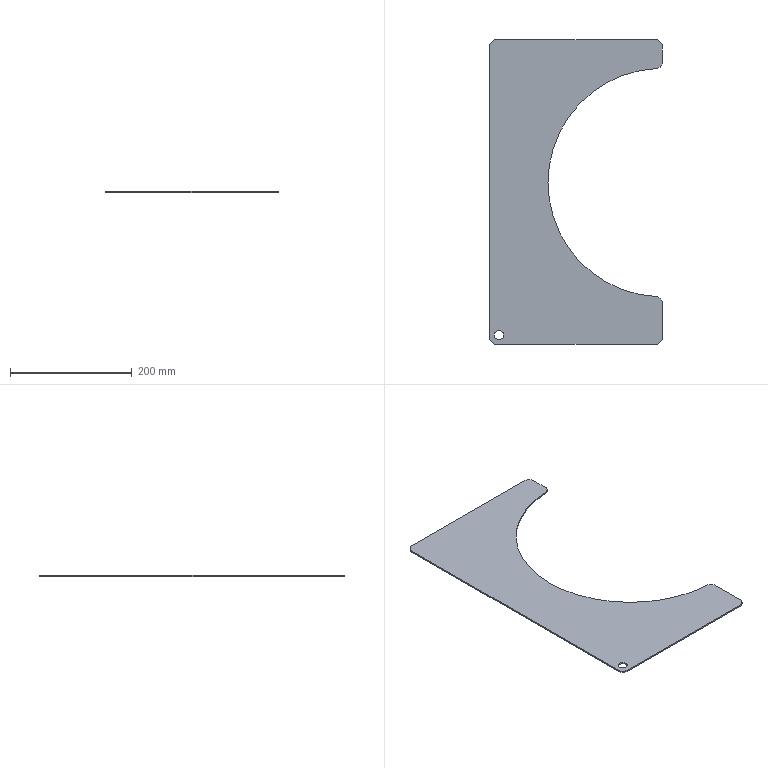Part | SolidWorks | features FlatPattern 1, SMBaseFlange 1, SheetMetal 1 | 1 solid | 17 faces | box 283 x 500 x 2.3 mm | volume 197741 mm3 | cylinder 10 | plane 7 | commonest cylinder face diameters 20 x6 15 x2 375 x2
STEP:
#1=CARTESIAN_POINT('',(7.5,-310.5,2.3));
#2=VERTEX_POINT('',#1);
#3=CARTESIAN_POINT('',(22.5,-310.5,2.3));
#4=VERTEX_POINT('',#3);
#5=CARTESIAN_POINT('',(15.,-310.5,2.3));
#6=DIRECTION('',(0.,0.,1.));
#7=DIRECTION('',(1.,0.,0.));
#8=AXIS2_PLACEMENT_3D('',#5,#6,#7);
#9=CIRCLE('',#8,7.5);
#10=EDGE_CURVE('',#2,#4,#9,.T.);
#11=ORIENTED_EDGE('',*,*,#10,.T.);
#12=CARTESIAN_POINT('',(22.5,-310.5,0.));
#13=VERTEX_POINT('',#12);
#14=CARTESIAN_POINT('',(22.5,-310.5,2.3));
#15=DIRECTION('',(0.,0.,-1.));
#16=VECTOR('',#15,1000.);
#17=LINE('',#14,#16);
#18=EDGE_CURVE('',#4,#13,#17,.T.);
#19=ORIENTED_EDGE('',*,*,#18,.T.);
#20=CARTESIAN_POINT('',(7.5,-310.5,0.));
#21=VERTEX_POINT('',#20);
#22=CARTESIAN_POINT('',(15.,-310.5,0.));
#23=DIRECTION('',(0.,0.,1.));
#24=DIRECTION('',(1.,0.,0.));
#25=AXIS2_PLACEMENT_3D('',#22,#23,#24);
#26=CIRCLE('',#25,7.5);
#27=EDGE_CURVE('',#21,#13,#26,.T.);
#28=ORIENTED_EDGE('',*,*,#27,.F.);
#29=CARTESIAN_POINT('',(7.5,-310.5,2.3));
#30=DIRECTION('',(0.,0.,-1.));
#31=VECTOR('',#30,1000.);
#32=LINE('',#29,#31);
#33=EDGE_CURVE('',#2,#21,#32,.T.);
#34=ORIENTED_EDGE('',*,*,#33,.F.);
#35=EDGE_LOOP('',(#11,#19,#28,#34));
#36=FACE_OUTER_BOUND('',#35,.T.);
#37=CARTESIAN_POINT('',(15.,-310.5,2.3));
#38=DIRECTION('',(0.,0.,-1.));
#39=DIRECTION('',(-1.,0.,0.));
#40=AXIS2_PLACEMENT_3D('',#37,#38,#39);
#41=CYLINDRICAL_SURFACE('',#40,7.5);
#42=ADVANCED_FACE('',(#36),#41,.F.);
#43=CARTESIAN_POINT('',(95.5,-60.,2.3));
#44=VERTEX_POINT('',#43);
#45=CARTESIAN_POINT('',(273.506,127.259,2.3));
#46=VERTEX_POINT('',#45);
#47=CARTESIAN_POINT('',(283.,-60.,2.3));
#48=DIRECTION('',(0.,0.,-1.));
#49=DIRECTION('',(1.,0.,0.));
#50=AXIS2_PLACEMENT_3D('',#47,#48,#49);
#51=CIRCLE('',#50,187.5);
#52=EDGE_CURVE('',#44,#46,#51,.T.);
#53=ORIENTED_EDGE('',*,*,#52,.F.);
#54=CARTESIAN_POINT('',(95.5,-60.,0.));
#55=VERTEX_POINT('',#54);
#56=CARTESIAN_POINT('',(95.5,-60.,2.3));
#57=DIRECTION('',(0.,0.,-1.));
#58=VECTOR('',#57,1000.);
#59=LINE('',#56,#58);
#60=EDGE_CURVE('',#44,#55,#59,.T.);
#61=ORIENTED_EDGE('',*,*,#60,.T.);
#62=CARTESIAN_POINT('',(273.506,127.259,0.));
#63=VERTEX_POINT('',#62);
#64=CARTESIAN_POINT('',(283.,-60.,0.));
#65=DIRECTION('',(0.,0.,-1.));
#66=DIRECTION('',(1.,0.,0.));
#67=AXIS2_PLACEMENT_3D('',#64,#65,#66);
#68=CIRCLE('',#67,187.5);
#69=EDGE_CURVE('',#55,#63,#68,.T.);
#70=ORIENTED_EDGE('',*,*,#69,.T.);
#71=CARTESIAN_POINT('',(273.506,127.259,2.3));
#72=DIRECTION('',(0.,0.,-1.));
#73=VECTOR('',#72,1000.);
#74=LINE('',#71,#73);
#75=EDGE_CURVE('',#46,#63,#74,.T.);
#76=ORIENTED_EDGE('',*,*,#75,.F.);
#77=EDGE_LOOP('',(#53,#61,#70,#76));
#78=FACE_OUTER_BOUND('',#77,.T.);
#79=CARTESIAN_POINT('',(283.,-60.,2.3));
#80=DIRECTION('',(0.,0.,-1.));
#81=DIRECTION('',(-1.,0.,0.));
#82=AXIS2_PLACEMENT_3D('',#79,#80,#81);
#83=CYLINDRICAL_SURFACE('',#82,187.5);
#84=ADVANCED_FACE('',(#78),#83,.F.);
#85=CARTESIAN_POINT('',(283.,-257.247,2.3));
#86=VERTEX_POINT('',#85);
#87=CARTESIAN_POINT('',(273.506,-247.259,2.3));
#88=VERTEX_POINT('',#87);
#89=CARTESIAN_POINT('',(273.,-257.247,2.3));
#90=DIRECTION('',(0.,0.,1.));
#91=DIRECTION('',(-1.,0.,0.));
#92=AXIS2_PLACEMENT_3D('',#89,#90,#91);
#93=CIRCLE('',#92,10.);
#94=EDGE_CURVE('',#86,#88,#93,.T.);
#95=ORIENTED_EDGE('',*,*,#94,.T.);
#96=CARTESIAN_POINT('',(283.,-60.,2.3));
#97=DIRECTION('',(0.,0.,-1.));
#98=DIRECTION('',(1.,0.,0.));
#99=AXIS2_PLACEMENT_3D('',#96,#97,#98);
#100=CIRCLE('',#99,187.5);
#101=EDGE_CURVE('',#88,#44,#100,.T.);
#102=ORIENTED_EDGE('',*,*,#101,.T.);
#103=ORIENTED_EDGE('',*,*,#52,.T.);
#104=CARTESIAN_POINT('',(283.,137.247,2.3));
#105=VERTEX_POINT('',#104);
#106=CARTESIAN_POINT('',(273.,137.247,2.3));
#107=DIRECTION('',(0.,0.,1.));
#108=DIRECTION('',(1.,0.,0.));
#109=AXIS2_PLACEMENT_3D('',#106,#107,#108);
#110=CIRCLE('',#109,10.);
#111=EDGE_CURVE('',#46,#105,#110,.T.);
#112=ORIENTED_EDGE('',*,*,#111,.T.);
#113=CARTESIAN_POINT('',(283.,164.5,2.3));
#114=VERTEX_POINT('',#113);
#115=CARTESIAN_POINT('',(283.,137.247,2.3));
#116=DIRECTION('',(0.,1.,0.));
#117=VECTOR('',#116,1000.);
#118=LINE('',#115,#117);
#119=EDGE_CURVE('',#105,#114,#118,.T.);
#120=ORIENTED_EDGE('',*,*,#119,.T.);
#121=CARTESIAN_POINT('',(273.,174.5,2.3));
#122=VERTEX_POINT('',#121);
#123=CARTESIAN_POINT('',(273.,164.5,2.3));
#124=DIRECTION('',(0.,0.,1.));
#125=DIRECTION('',(-1.,0.,0.));
#126=AXIS2_PLACEMENT_3D('',#123,#124,#125);
#127=CIRCLE('',#126,10.);
#128=EDGE_CURVE('',#114,#122,#127,.T.);
#129=ORIENTED_EDGE('',*,*,#128,.T.);
#130=CARTESIAN_POINT('',(10.,174.5,2.3));
#131=VERTEX_POINT('',#130);
#132=CARTESIAN_POINT('',(10.,174.5,2.3));
#133=DIRECTION('',(-1.,0.,0.));
#134=VECTOR('',#133,1000.);
#135=LINE('',#132,#134);
#136=EDGE_CURVE('',#122,#131,#135,.T.);
#137=ORIENTED_EDGE('',*,*,#136,.T.);
#138=CARTESIAN_POINT('',(0.,164.5,2.3));
#139=VERTEX_POINT('',#138);
#140=CARTESIAN_POINT('',(10.,164.5,2.3));
#141=DIRECTION('',(0.,0.,1.));
#142=DIRECTION('',(-1.,0.,0.));
#143=AXIS2_PLACEMENT_3D('',#140,#141,#142);
#144=CIRCLE('',#143,10.);
#145=EDGE_CURVE('',#131,#139,#144,.T.);
#146=ORIENTED_EDGE('',*,*,#145,.T.);
#147=CARTESIAN_POINT('',(0.,-315.5,2.3));
#148=VERTEX_POINT('',#147);
#149=CARTESIAN_POINT('',(0.,-315.5,2.3));
#150=DIRECTION('',(0.,-1.,0.));
#151=VECTOR('',#150,1000.);
#152=LINE('',#149,#151);
#153=EDGE_CURVE('',#139,#148,#152,.T.);
#154=ORIENTED_EDGE('',*,*,#153,.T.);
#155=CARTESIAN_POINT('',(10.,-325.5,2.3));
#156=VERTEX_POINT('',#155);
#157=CARTESIAN_POINT('',(10.,-315.5,2.3));
#158=DIRECTION('',(0.,0.,1.));
#159=DIRECTION('',(-1.,0.,0.));
#160=AXIS2_PLACEMENT_3D('',#157,#158,#159);
#161=CIRCLE('',#160,10.);
#162=EDGE_CURVE('',#148,#156,#161,.T.);
#163=ORIENTED_EDGE('',*,*,#162,.T.);
#164=CARTESIAN_POINT('',(273.,-325.5,2.3));
#165=VERTEX_POINT('',#164);
#166=CARTESIAN_POINT('',(10.,-325.5,2.3));
#167=DIRECTION('',(1.,0.,0.));
#168=VECTOR('',#167,1000.);
#169=LINE('',#166,#168);
#170=EDGE_CURVE('',#156,#165,#169,.T.);
#171=ORIENTED_EDGE('',*,*,#170,.T.);
#172=CARTESIAN_POINT('',(283.,-315.5,2.3));
#173=VERTEX_POINT('',#172);
#174=CARTESIAN_POINT('',(273.,-315.5,2.3));
#175=DIRECTION('',(0.,0.,1.));
#176=DIRECTION('',(1.,0.,0.));
#177=AXIS2_PLACEMENT_3D('',#174,#175,#176);
#178=CIRCLE('',#177,10.);
#179=EDGE_CURVE('',#165,#173,#178,.T.);
#180=ORIENTED_EDGE('',*,*,#179,.T.);
#181=CARTESIAN_POINT('',(283.,-315.5,2.3));
#182=DIRECTION('',(0.,1.,0.));
#183=VECTOR('',#182,1000.);
#184=LINE('',#181,#183);
#185=EDGE_CURVE('',#173,#86,#184,.T.);
#186=ORIENTED_EDGE('',*,*,#185,.T.);
#187=EDGE_LOOP('',(#95,#102,#103,#112,#120,#129,#137,#146,#154,#163,#171,#180,#186));
#188=FACE_OUTER_BOUND('',#187,.T.);
#189=ORIENTED_EDGE('',*,*,#10,.F.);
#190=CARTESIAN_POINT('',(15.,-310.5,2.3));
#191=DIRECTION('',(0.,0.,1.));
#192=DIRECTION('',(1.,0.,0.));
#193=AXIS2_PLACEMENT_3D('',#190,#191,#192);
#194=CIRCLE('',#193,7.5);
#195=EDGE_CURVE('',#4,#2,#194,.T.);
#196=ORIENTED_EDGE('',*,*,#195,.F.);
#197=EDGE_LOOP('',(#189,#196));
#198=FACE_BOUND('',#197,.T.);
#199=CARTESIAN_POINT('',(273.,-257.247,2.3));
#200=DIRECTION('',(0.,0.,-1.));
#201=DIRECTION('',(-1.,0.,0.));
#202=AXIS2_PLACEMENT_3D('',#199,#200,#201);
#203=PLANE('',#202);
#204=ADVANCED_FACE('',(#188,#198),#203,.F.);
#205=CARTESIAN_POINT('',(283.,-257.247,0.));
#206=VERTEX_POINT('',#205);
#207=CARTESIAN_POINT('',(273.506,-247.259,0.));
#208=VERTEX_POINT('',#207);
#209=CARTESIAN_POINT('',(273.,-257.247,0.));
#210=DIRECTION('',(0.,0.,1.));
#211=DIRECTION('',(-1.,0.,0.));
#212=AXIS2_PLACEMENT_3D('',#209,#210,#211);
#213=CIRCLE('',#212,10.);
#214=EDGE_CURVE('',#206,#208,#213,.T.);
#215=ORIENTED_EDGE('',*,*,#214,.F.);
#216=CARTESIAN_POINT('',(283.,-315.5,0.));
#217=VERTEX_POINT('',#216);
#218=CARTESIAN_POINT('',(283.,-315.5,0.));
#219=DIRECTION('',(0.,1.,0.));
#220=VECTOR('',#219,1000.);
#221=LINE('',#218,#220);
#222=EDGE_CURVE('',#217,#206,#221,.T.);
#223=ORIENTED_EDGE('',*,*,#222,.F.);
#224=CARTESIAN_POINT('',(273.,-325.5,0.));
#225=VERTEX_POINT('',#224);
#226=CARTESIAN_POINT('',(273.,-315.5,0.));
#227=DIRECTION('',(0.,0.,1.));
#228=DIRECTION('',(1.,0.,0.));
#229=AXIS2_PLACEMENT_3D('',#226,#227,#228);
#230=CIRCLE('',#229,10.);
#231=EDGE_CURVE('',#225,#217,#230,.T.);
#232=ORIENTED_EDGE('',*,*,#231,.F.);
#233=CARTESIAN_POINT('',(10.,-325.5,0.));
#234=VERTEX_POINT('',#233);
#235=CARTESIAN_POINT('',(10.,-325.5,0.));
#236=DIRECTION('',(1.,0.,0.));
#237=VECTOR('',#236,1000.);
#238=LINE('',#235,#237);
#239=EDGE_CURVE('',#234,#225,#238,.T.);
#240=ORIENTED_EDGE('',*,*,#239,.F.);
#241=CARTESIAN_POINT('',(0.,-315.5,0.));
#242=VERTEX_POINT('',#241);
#243=CARTESIAN_POINT('',(10.,-315.5,0.));
#244=DIRECTION('',(0.,0.,1.));
#245=DIRECTION('',(-1.,0.,0.));
#246=AXIS2_PLACEMENT_3D('',#243,#244,#245);
#247=CIRCLE('',#246,10.);
#248=EDGE_CURVE('',#242,#234,#247,.T.);
#249=ORIENTED_EDGE('',*,*,#248,.F.);
#250=CARTESIAN_POINT('',(0.,164.5,0.));
#251=VERTEX_POINT('',#250);
#252=CARTESIAN_POINT('',(0.,-315.5,0.));
#253=DIRECTION('',(0.,-1.,0.));
#254=VECTOR('',#253,1000.);
#255=LINE('',#252,#254);
#256=EDGE_CURVE('',#251,#242,#255,.T.);
#257=ORIENTED_EDGE('',*,*,#256,.F.);
#258=CARTESIAN_POINT('',(10.,174.5,0.));
#259=VERTEX_POINT('',#258);
#260=CARTESIAN_POINT('',(10.,164.5,0.));
#261=DIRECTION('',(0.,0.,1.));
#262=DIRECTION('',(-1.,0.,0.));
#263=AXIS2_PLACEMENT_3D('',#260,#261,#262);
#264=CIRCLE('',#263,10.);
#265=EDGE_CURVE('',#259,#251,#264,.T.);
#266=ORIENTED_EDGE('',*,*,#265,.F.);
#267=CARTESIAN_POINT('',(273.,174.5,0.));
#268=VERTEX_POINT('',#267);
#269=CARTESIAN_POINT('',(10.,174.5,0.));
#270=DIRECTION('',(-1.,0.,0.));
#271=VECTOR('',#270,1000.);
#272=LINE('',#269,#271);
#273=EDGE_CURVE('',#268,#259,#272,.T.);
#274=ORIENTED_EDGE('',*,*,#273,.F.);
#275=CARTESIAN_POINT('',(283.,164.5,0.));
#276=VERTEX_POINT('',#275);
#277=CARTESIAN_POINT('',(273.,164.5,0.));
#278=DIRECTION('',(0.,0.,1.));
#279=DIRECTION('',(-1.,0.,0.));
#280=AXIS2_PLACEMENT_3D('',#277,#278,#279);
#281=CIRCLE('',#280,10.);
#282=EDGE_CURVE('',#276,#268,#281,.T.);
#283=ORIENTED_EDGE('',*,*,#282,.F.);
#284=CARTESIAN_POINT('',(283.,137.247,0.));
#285=VERTEX_POINT('',#284);
#286=CARTESIAN_POINT('',(283.,137.247,0.));
#287=DIRECTION('',(0.,1.,0.));
#288=VECTOR('',#287,1000.);
#289=LINE('',#286,#288);
#290=EDGE_CURVE('',#285,#276,#289,.T.);
#291=ORIENTED_EDGE('',*,*,#290,.F.);
#292=CARTESIAN_POINT('',(273.,137.247,0.));
#293=DIRECTION('',(0.,0.,1.));
#294=DIRECTION('',(1.,0.,0.));
#295=AXIS2_PLACEMENT_3D('',#292,#293,#294);
#296=CIRCLE('',#295,10.);
#297=EDGE_CURVE('',#63,#285,#296,.T.);
#298=ORIENTED_EDGE('',*,*,#297,.F.);
#299=ORIENTED_EDGE('',*,*,#69,.F.);
#300=CARTESIAN_POINT('',(283.,-60.,0.));
#301=DIRECTION('',(0.,0.,-1.));
#302=DIRECTION('',(1.,0.,0.));
#303=AXIS2_PLACEMENT_3D('',#300,#301,#302);
#304=CIRCLE('',#303,187.5);
#305=EDGE_CURVE('',#208,#55,#304,.T.);
#306=ORIENTED_EDGE('',*,*,#305,.F.);
#307=EDGE_LOOP('',(#215,#223,#232,#240,#249,#257,#266,#274,#283,#291,#298,#299,#306));
#308=FACE_OUTER_BOUND('',#307,.T.);
#309=ORIENTED_EDGE('',*,*,#27,.T.);
#310=CARTESIAN_POINT('',(15.,-310.5,0.));
#311=DIRECTION('',(0.,0.,1.));
#312=DIRECTION('',(1.,0.,0.));
#313=AXIS2_PLACEMENT_3D('',#310,#311,#312);
#314=CIRCLE('',#313,7.5);
#315=EDGE_CURVE('',#13,#21,#314,.T.);
#316=ORIENTED_EDGE('',*,*,#315,.T.);
#317=EDGE_LOOP('',(#309,#316));
#318=FACE_BOUND('',#317,.T.);
#319=CARTESIAN_POINT('',(273.,-257.247,0.));
#320=DIRECTION('',(0.,0.,-1.));
#321=DIRECTION('',(-1.,0.,0.));
#322=AXIS2_PLACEMENT_3D('',#319,#320,#321);
#323=PLANE('',#322);
#324=ADVANCED_FACE('',(#308,#318),#323,.T.);
#325=ORIENTED_EDGE('',*,*,#214,.T.);
#326=CARTESIAN_POINT('',(273.506,-247.259,2.3));
#327=DIRECTION('',(0.,0.,-1.));
#328=VECTOR('',#327,1000.);
#329=LINE('',#326,#328);
#330=EDGE_CURVE('',#88,#208,#329,.T.);
#331=ORIENTED_EDGE('',*,*,#330,.F.);
#332=ORIENTED_EDGE('',*,*,#94,.F.);
#333=CARTESIAN_POINT('',(283.,-257.247,2.3));
#334=DIRECTION('',(0.,0.,-1.));
#335=VECTOR('',#334,1000.);
#336=LINE('',#333,#335);
#337=EDGE_CURVE('',#86,#206,#336,.T.);
#338=ORIENTED_EDGE('',*,*,#337,.T.);
#339=EDGE_LOOP('',(#325,#331,#332,#338));
#340=FACE_OUTER_BOUND('',#339,.T.);
#341=CARTESIAN_POINT('',(273.,-257.247,2.3));
#342=DIRECTION('',(0.,0.,-1.));
#343=DIRECTION('',(-1.,0.,0.));
#344=AXIS2_PLACEMENT_3D('',#341,#342,#343);
#345=CYLINDRICAL_SURFACE('',#344,10.);
#346=ADVANCED_FACE('',(#340),#345,.T.);
#347=ORIENTED_EDGE('',*,*,#60,.F.);
#348=ORIENTED_EDGE('',*,*,#101,.F.);
#349=ORIENTED_EDGE('',*,*,#330,.T.);
#350=ORIENTED_EDGE('',*,*,#305,.T.);
#351=EDGE_LOOP('',(#347,#348,#349,#350));
#352=FACE_OUTER_BOUND('',#351,.T.);
#353=CARTESIAN_POINT('',(283.,-60.,2.3));
#354=DIRECTION('',(0.,0.,-1.));
#355=DIRECTION('',(-1.,0.,0.));
#356=AXIS2_PLACEMENT_3D('',#353,#354,#355);
#357=CYLINDRICAL_SURFACE('',#356,187.5);
#358=ADVANCED_FACE('',(#352),#357,.F.);
#359=ORIENTED_EDGE('',*,*,#297,.T.);
#360=CARTESIAN_POINT('',(283.,137.247,2.3));
#361=DIRECTION('',(0.,0.,-1.));
#362=VECTOR('',#361,1000.);
#363=LINE('',#360,#362);
#364=EDGE_CURVE('',#105,#285,#363,.T.);
#365=ORIENTED_EDGE('',*,*,#364,.F.);
#366=ORIENTED_EDGE('',*,*,#111,.F.);
#367=ORIENTED_EDGE('',*,*,#75,.T.);
#368=EDGE_LOOP('',(#359,#365,#366,#367));
#369=FACE_OUTER_BOUND('',#368,.T.);
#370=CARTESIAN_POINT('',(273.,137.247,2.3));
#371=DIRECTION('',(0.,0.,-1.));
#372=DIRECTION('',(-1.,0.,0.));
#373=AXIS2_PLACEMENT_3D('',#370,#371,#372);
#374=CYLINDRICAL_SURFACE('',#373,10.);
#375=ADVANCED_FACE('',(#369),#374,.T.);
#376=ORIENTED_EDGE('',*,*,#290,.T.);
#377=CARTESIAN_POINT('',(283.,164.5,2.3));
#378=DIRECTION('',(0.,0.,-1.));
#379=VECTOR('',#378,1000.);
#380=LINE('',#377,#379);
#381=EDGE_CURVE('',#114,#276,#380,.T.);
#382=ORIENTED_EDGE('',*,*,#381,.F.);
#383=ORIENTED_EDGE('',*,*,#119,.F.);
#384=ORIENTED_EDGE('',*,*,#364,.T.);
#385=EDGE_LOOP('',(#376,#382,#383,#384));
#386=FACE_OUTER_BOUND('',#385,.T.);
#387=CARTESIAN_POINT('',(283.,137.247,2.3));
#388=DIRECTION('',(-1.,0.,0.));
#389=DIRECTION('',(0.,0.,1.));
#390=AXIS2_PLACEMENT_3D('',#387,#388,#389);
#391=PLANE('',#390);
#392=ADVANCED_FACE('',(#386),#391,.F.);
#393=ORIENTED_EDGE('',*,*,#282,.T.);
#394=CARTESIAN_POINT('',(273.,174.5,2.3));
#395=DIRECTION('',(0.,0.,-1.));
#396=VECTOR('',#395,1000.);
#397=LINE('',#394,#396);
#398=EDGE_CURVE('',#122,#268,#397,.T.);
#399=ORIENTED_EDGE('',*,*,#398,.F.);
#400=ORIENTED_EDGE('',*,*,#128,.F.);
#401=ORIENTED_EDGE('',*,*,#381,.T.);
#402=EDGE_LOOP('',(#393,#399,#400,#401));
#403=FACE_OUTER_BOUND('',#402,.T.);
#404=CARTESIAN_POINT('',(273.,164.5,2.3));
#405=DIRECTION('',(0.,0.,-1.));
#406=DIRECTION('',(-1.,0.,0.));
#407=AXIS2_PLACEMENT_3D('',#404,#405,#406);
#408=CYLINDRICAL_SURFACE('',#407,10.);
#409=ADVANCED_FACE('',(#403),#408,.T.);
#410=ORIENTED_EDGE('',*,*,#273,.T.);
#411=CARTESIAN_POINT('',(10.,174.5,2.3));
#412=DIRECTION('',(0.,0.,-1.));
#413=VECTOR('',#412,1000.);
#414=LINE('',#411,#413);
#415=EDGE_CURVE('',#131,#259,#414,.T.);
#416=ORIENTED_EDGE('',*,*,#415,.F.);
#417=ORIENTED_EDGE('',*,*,#136,.F.);
#418=ORIENTED_EDGE('',*,*,#398,.T.);
#419=EDGE_LOOP('',(#410,#416,#417,#418));
#420=FACE_OUTER_BOUND('',#419,.T.);
#421=CARTESIAN_POINT('',(10.,174.5,2.3));
#422=DIRECTION('',(0.,-1.,0.));
#423=DIRECTION('',(0.,0.,-1.));
#424=AXIS2_PLACEMENT_3D('',#421,#422,#423);
#425=PLANE('',#424);
#426=ADVANCED_FACE('',(#420),#425,.F.);
#427=ORIENTED_EDGE('',*,*,#265,.T.);
#428=CARTESIAN_POINT('',(0.,164.5,2.3));
#429=DIRECTION('',(0.,0.,-1.));
#430=VECTOR('',#429,1000.);
#431=LINE('',#428,#430);
#432=EDGE_CURVE('',#139,#251,#431,.T.);
#433=ORIENTED_EDGE('',*,*,#432,.F.);
#434=ORIENTED_EDGE('',*,*,#145,.F.);
#435=ORIENTED_EDGE('',*,*,#415,.T.);
#436=EDGE_LOOP('',(#427,#433,#434,#435));
#437=FACE_OUTER_BOUND('',#436,.T.);
#438=CARTESIAN_POINT('',(10.,164.5,2.3));
#439=DIRECTION('',(0.,0.,-1.));
#440=DIRECTION('',(-1.,0.,0.));
#441=AXIS2_PLACEMENT_3D('',#438,#439,#440);
#442=CYLINDRICAL_SURFACE('',#441,10.);
#443=ADVANCED_FACE('',(#437),#442,.T.);
#444=ORIENTED_EDGE('',*,*,#256,.T.);
#445=CARTESIAN_POINT('',(0.,-315.5,2.3));
#446=DIRECTION('',(0.,0.,-1.));
#447=VECTOR('',#446,1000.);
#448=LINE('',#445,#447);
#449=EDGE_CURVE('',#148,#242,#448,.T.);
#450=ORIENTED_EDGE('',*,*,#449,.F.);
#451=ORIENTED_EDGE('',*,*,#153,.F.);
#452=ORIENTED_EDGE('',*,*,#432,.T.);
#453=EDGE_LOOP('',(#444,#450,#451,#452));
#454=FACE_OUTER_BOUND('',#453,.T.);
#455=CARTESIAN_POINT('',(0.,-315.5,2.3));
#456=DIRECTION('',(1.,0.,0.));
#457=DIRECTION('',(0.,1.,0.));
#458=AXIS2_PLACEMENT_3D('',#455,#456,#457);
#459=PLANE('',#458);
#460=ADVANCED_FACE('',(#454),#459,.F.);
#461=ORIENTED_EDGE('',*,*,#248,.T.);
#462=CARTESIAN_POINT('',(10.,-325.5,2.3));
#463=DIRECTION('',(0.,0.,-1.));
#464=VECTOR('',#463,1000.);
#465=LINE('',#462,#464);
#466=EDGE_CURVE('',#156,#234,#465,.T.);
#467=ORIENTED_EDGE('',*,*,#466,.F.);
#468=ORIENTED_EDGE('',*,*,#162,.F.);
#469=ORIENTED_EDGE('',*,*,#449,.T.);
#470=EDGE_LOOP('',(#461,#467,#468,#469));
#471=FACE_OUTER_BOUND('',#470,.T.);
#472=CARTESIAN_POINT('',(10.,-315.5,2.3));
#473=DIRECTION('',(0.,0.,-1.));
#474=DIRECTION('',(-1.,0.,0.));
#475=AXIS2_PLACEMENT_3D('',#472,#473,#474);
#476=CYLINDRICAL_SURFACE('',#475,10.);
#477=ADVANCED_FACE('',(#471),#476,.T.);
#478=ORIENTED_EDGE('',*,*,#239,.T.);
#479=CARTESIAN_POINT('',(273.,-325.5,2.3));
#480=DIRECTION('',(0.,0.,-1.));
#481=VECTOR('',#480,1000.);
#482=LINE('',#479,#481);
#483=EDGE_CURVE('',#165,#225,#482,.T.);
#484=ORIENTED_EDGE('',*,*,#483,.F.);
#485=ORIENTED_EDGE('',*,*,#170,.F.);
#486=ORIENTED_EDGE('',*,*,#466,.T.);
#487=EDGE_LOOP('',(#478,#484,#485,#486));
#488=FACE_OUTER_BOUND('',#487,.T.);
#489=CARTESIAN_POINT('',(10.,-325.5,2.3));
#490=DIRECTION('',(0.,1.,0.));
#491=DIRECTION('',(0.,0.,1.));
#492=AXIS2_PLACEMENT_3D('',#489,#490,#491);
#493=PLANE('',#492);
#494=ADVANCED_FACE('',(#488),#493,.F.);
#495=ORIENTED_EDGE('',*,*,#231,.T.);
#496=CARTESIAN_POINT('',(283.,-315.5,2.3));
#497=DIRECTION('',(0.,0.,-1.));
#498=VECTOR('',#497,1000.);
#499=LINE('',#496,#498);
#500=EDGE_CURVE('',#173,#217,#499,.T.);
#501=ORIENTED_EDGE('',*,*,#500,.F.);
#502=ORIENTED_EDGE('',*,*,#179,.F.);
#503=ORIENTED_EDGE('',*,*,#483,.T.);
#504=EDGE_LOOP('',(#495,#501,#502,#503));
#505=FACE_OUTER_BOUND('',#504,.T.);
#506=CARTESIAN_POINT('',(273.,-315.5,2.3));
#507=DIRECTION('',(0.,0.,-1.));
#508=DIRECTION('',(-1.,0.,0.));
#509=AXIS2_PLACEMENT_3D('',#506,#507,#508);
#510=CYLINDRICAL_SURFACE('',#509,10.);
#511=ADVANCED_FACE('',(#505),#510,.T.);
#512=ORIENTED_EDGE('',*,*,#222,.T.);
#513=ORIENTED_EDGE('',*,*,#337,.F.);
#514=ORIENTED_EDGE('',*,*,#185,.F.);
#515=ORIENTED_EDGE('',*,*,#500,.T.);
#516=EDGE_LOOP('',(#512,#513,#514,#515));
#517=FACE_OUTER_BOUND('',#516,.T.);
#518=CARTESIAN_POINT('',(283.,-315.5,2.3));
#519=DIRECTION('',(-1.,0.,0.));
#520=DIRECTION('',(0.,0.,1.));
#521=AXIS2_PLACEMENT_3D('',#518,#519,#520);
#522=PLANE('',#521);
#523=ADVANCED_FACE('',(#517),#522,.F.);
#524=ORIENTED_EDGE('',*,*,#18,.F.);
#525=ORIENTED_EDGE('',*,*,#195,.T.);
#526=ORIENTED_EDGE('',*,*,#33,.T.);
#527=ORIENTED_EDGE('',*,*,#315,.F.);
#528=EDGE_LOOP('',(#524,#525,#526,#527));
#529=FACE_OUTER_BOUND('',#528,.T.);
#530=CARTESIAN_POINT('',(15.,-310.5,2.3));
#531=DIRECTION('',(0.,0.,-1.));
#532=DIRECTION('',(-1.,0.,0.));
#533=AXIS2_PLACEMENT_3D('',#530,#531,#532);
#534=CYLINDRICAL_SURFACE('',#533,7.5);
#535=ADVANCED_FACE('',(#529),#534,.F.);
#536=CLOSED_SHELL('',(#42,#84,#204,#324,#346,#358,#375,#392,#409,#426,#443,#460,#477,#494,#511,#523,#535));
#537=MANIFOLD_SOLID_BREP('',#536);
#538=CARTESIAN_POINT('',(0.,0.,0.));
#539=DIRECTION('',(0.,0.,1.));
#540=DIRECTION('',(1.,0.,0.));
#541=AXIS2_PLACEMENT_3D('',#538,#539,#540);
#542=(LENGTH_UNIT()NAMED_UNIT(*)SI_UNIT(.MILLI.,.METRE.));
#543=UNCERTAINTY_MEASURE_WITH_UNIT(LENGTH_MEASURE(0.00001),#542,'','');
#544=(NAMED_UNIT(*)PLANE_ANGLE_UNIT()SI_UNIT($,.RADIAN.));
#545=(NAMED_UNIT(*)SI_UNIT($,.STERADIAN.)SOLID_ANGLE_UNIT());
#546=(GEOMETRIC_REPRESENTATION_CONTEXT(3)GLOBAL_UNCERTAINTY_ASSIGNED_CONTEXT((#543))GLOBAL_UNIT_ASSIGNED_CONTEXT((#542,#544,#545))REPRESENTATION_CONTEXT('',''));
#547=ADVANCED_BREP_SHAPE_REPRESENTATION('',(#537,#541),#546);